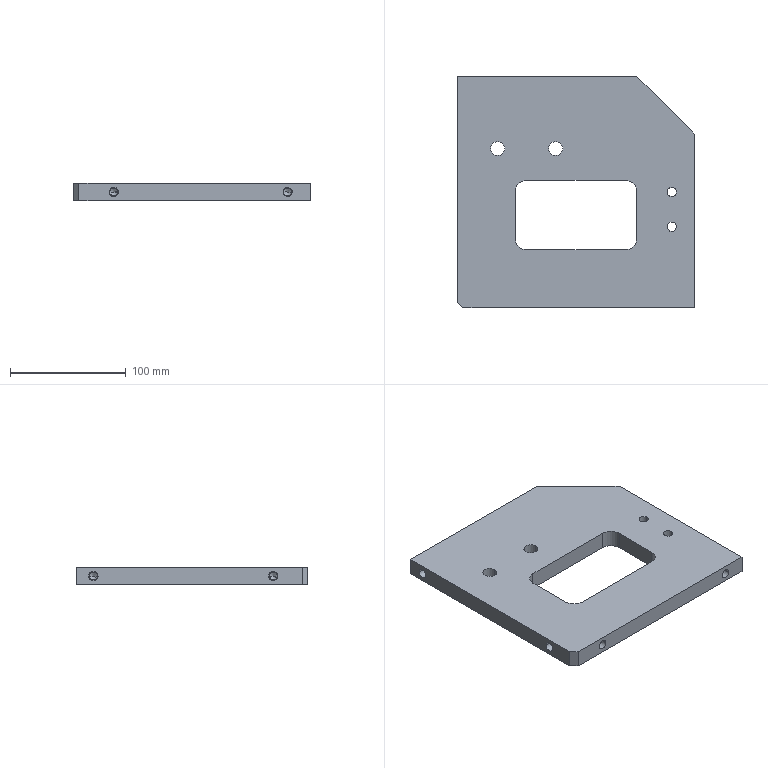Part | STEP file | J453-EBZ05-03-04 | 1 solid | 59 faces | box 205 x 200 x 15 mm | volume 493517 mm3 | cylinder 32 | plane 17 | cone 10 | commonest cylinder face diameters 8 x12 6.9 x8 12 x4 20 x4 5.1 x2 6 x2